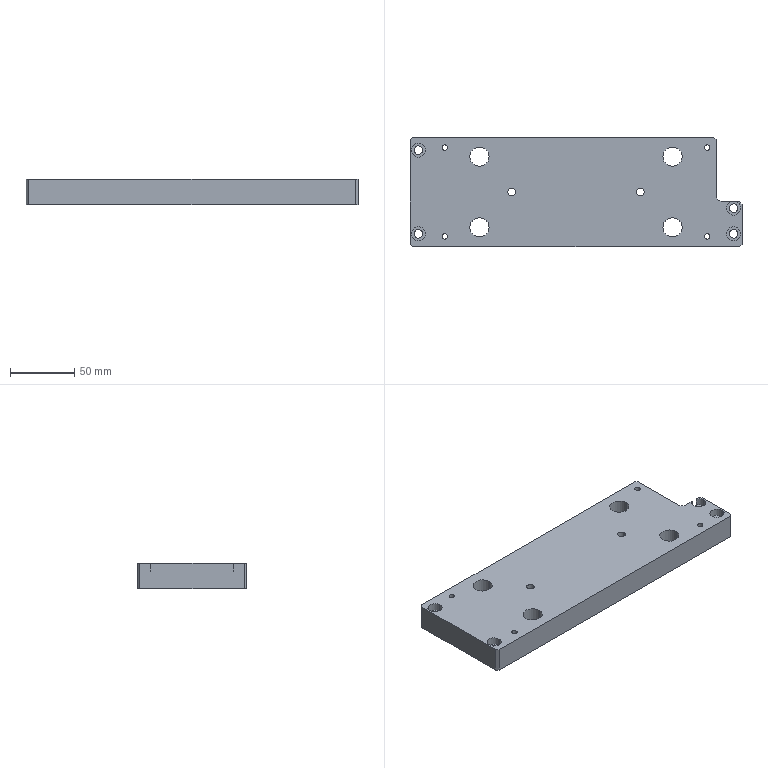Part | STEP file | PN_0024 | 1 solid | 55 faces | box 258 x 85 x 19.5 mm | volume 387959 mm3 | cylinder 38 | plane 17 | commonest cylinder face diameters 11 x9 4.2 x8 6.6 x8 15 x8 6 x4 10 x1